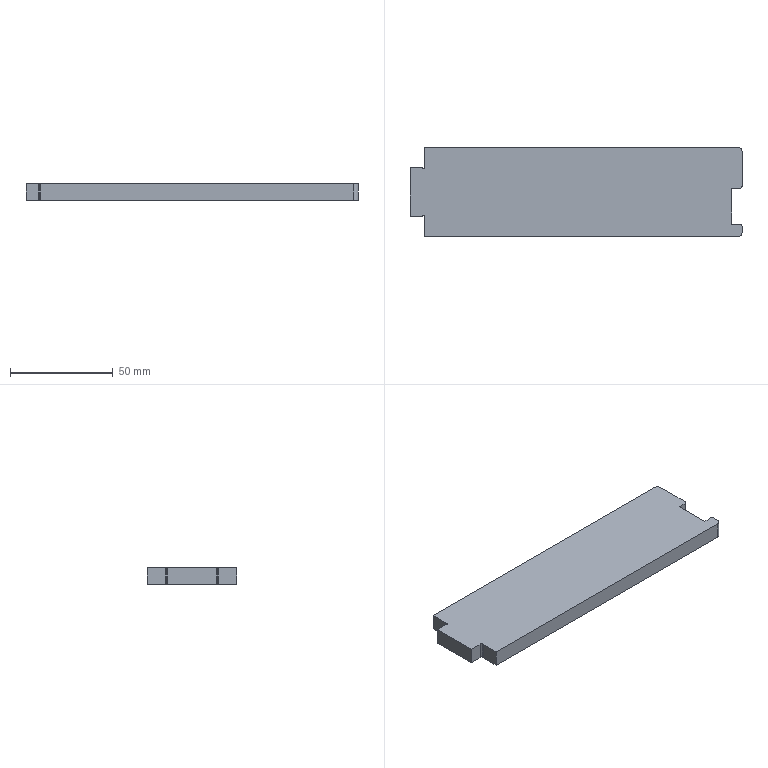Part | SolidWorks | features Fillet 2, FlatPattern 1, ICE 1, SMBaseFlange 1, SheetMetal 1 | 1 solid | 24 faces | box 161.8 x 43.5 x 8 mm | volume 54464 mm3 | plane 14 | cylinder 10 | commonest cylinder face diameters 2 x6 1 x2 4 x2
STEP:
#1=CARTESIAN_POINT('',(-162.8,318.921,0.));
#2=VERTEX_POINT('',#1);
#3=CARTESIAN_POINT('',(-162.8,310.,0.));
#4=VERTEX_POINT('',#3);
#5=CARTESIAN_POINT('',(-162.8,320.,0.));
#6=DIRECTION('',(0.,-1.,0.));
#7=VECTOR('',#6,1000.);
#8=LINE('',#5,#7);
#9=EDGE_CURVE('',#2,#4,#8,.T.);
#10=ORIENTED_EDGE('',*,*,#9,.F.);
#11=CARTESIAN_POINT('',(-162.8,318.921,-8.));
#12=VERTEX_POINT('',#11);
#13=CARTESIAN_POINT('',(-162.8,318.921,-8.));
#14=DIRECTION('',(0.,0.,-1.));
#15=VECTOR('',#14,1000.);
#16=LINE('',#13,#15);
#17=EDGE_CURVE('',#2,#12,#16,.T.);
#18=ORIENTED_EDGE('',*,*,#17,.T.);
#19=CARTESIAN_POINT('',(-162.8,310.,-8.));
#20=VERTEX_POINT('',#19);
#21=CARTESIAN_POINT('',(-162.8,320.,-8.));
#22=DIRECTION('',(0.,-1.,0.));
#23=VECTOR('',#22,1000.);
#24=LINE('',#21,#23);
#25=EDGE_CURVE('',#12,#20,#24,.T.);
#26=ORIENTED_EDGE('',*,*,#25,.T.);
#27=CARTESIAN_POINT('',(-162.8,310.,-8.));
#28=DIRECTION('',(0.,0.,1.));
#29=VECTOR('',#28,1000.);
#30=LINE('',#27,#29);
#31=EDGE_CURVE('',#20,#4,#30,.T.);
#32=ORIENTED_EDGE('',*,*,#31,.T.);
#33=EDGE_LOOP('',(#10,#18,#26,#32));
#34=FACE_OUTER_BOUND('',#33,.T.);
#35=CARTESIAN_POINT('',(-162.8,320.,-8.));
#36=DIRECTION('',(-1.,0.,0.));
#37=DIRECTION('',(0.,0.,1.));
#38=AXIS2_PLACEMENT_3D('',#35,#36,#37);
#39=PLANE('',#38);
#40=ADVANCED_FACE('',(#34),#39,.T.);
#41=CARTESIAN_POINT('',(-169.8,320.,-8.));
#42=VERTEX_POINT('',#41);
#43=CARTESIAN_POINT('',(-163.879,320.,-8.));
#44=VERTEX_POINT('',#43);
#45=CARTESIAN_POINT('',(-162.8,320.,-8.));
#46=DIRECTION('',(1.,0.,0.));
#47=VECTOR('',#46,1000.);
#48=LINE('',#45,#47);
#49=EDGE_CURVE('',#42,#44,#48,.T.);
#50=ORIENTED_EDGE('',*,*,#49,.T.);
#51=CARTESIAN_POINT('',(-163.879,320.,0.));
#52=VERTEX_POINT('',#51);
#53=CARTESIAN_POINT('',(-163.879,320.,-8.));
#54=DIRECTION('',(0.,0.,1.));
#55=VECTOR('',#54,1000.);
#56=LINE('',#53,#55);
#57=EDGE_CURVE('',#44,#52,#56,.T.);
#58=ORIENTED_EDGE('',*,*,#57,.T.);
#59=CARTESIAN_POINT('',(-169.8,320.,0.));
#60=VERTEX_POINT('',#59);
#61=CARTESIAN_POINT('',(-162.8,320.,0.));
#62=DIRECTION('',(1.,0.,0.));
#63=VECTOR('',#62,1000.);
#64=LINE('',#61,#63);
#65=EDGE_CURVE('',#60,#52,#64,.T.);
#66=ORIENTED_EDGE('',*,*,#65,.F.);
#67=CARTESIAN_POINT('',(-169.8,320.,-8.));
#68=DIRECTION('',(0.,0.,1.));
#69=VECTOR('',#68,1000.);
#70=LINE('',#67,#69);
#71=EDGE_CURVE('',#42,#60,#70,.T.);
#72=ORIENTED_EDGE('',*,*,#71,.F.);
#73=EDGE_LOOP('',(#50,#58,#66,#72));
#74=FACE_OUTER_BOUND('',#73,.T.);
#75=CARTESIAN_POINT('',(-162.8,320.,-8.));
#76=DIRECTION('',(0.,-1.,0.));
#77=DIRECTION('',(0.,0.,-1.));
#78=AXIS2_PLACEMENT_3D('',#75,#76,#77);
#79=PLANE('',#78);
#80=ADVANCED_FACE('',(#74),#79,.T.);
#81=CARTESIAN_POINT('',(-163.879,343.5,0.));
#82=VERTEX_POINT('',#81);
#83=CARTESIAN_POINT('',(-169.8,343.5,0.));
#84=VERTEX_POINT('',#83);
#85=CARTESIAN_POINT('',(-169.8,343.5,0.));
#86=DIRECTION('',(-1.,0.,0.));
#87=VECTOR('',#86,1000.);
#88=LINE('',#85,#87);
#89=EDGE_CURVE('',#82,#84,#88,.T.);
#90=ORIENTED_EDGE('',*,*,#89,.F.);
#91=CARTESIAN_POINT('',(-163.879,343.5,-8.));
#92=VERTEX_POINT('',#91);
#93=CARTESIAN_POINT('',(-163.879,343.5,-8.));
#94=DIRECTION('',(0.,0.,-1.));
#95=VECTOR('',#94,1000.);
#96=LINE('',#93,#95);
#97=EDGE_CURVE('',#82,#92,#96,.T.);
#98=ORIENTED_EDGE('',*,*,#97,.T.);
#99=CARTESIAN_POINT('',(-169.8,343.5,-8.));
#100=VERTEX_POINT('',#99);
#101=CARTESIAN_POINT('',(-169.8,343.5,-8.));
#102=DIRECTION('',(-1.,0.,0.));
#103=VECTOR('',#102,1000.);
#104=LINE('',#101,#103);
#105=EDGE_CURVE('',#92,#100,#104,.T.);
#106=ORIENTED_EDGE('',*,*,#105,.T.);
#107=CARTESIAN_POINT('',(-169.8,343.5,-8.));
#108=DIRECTION('',(0.,0.,1.));
#109=VECTOR('',#108,1000.);
#110=LINE('',#107,#109);
#111=EDGE_CURVE('',#100,#84,#110,.T.);
#112=ORIENTED_EDGE('',*,*,#111,.T.);
#113=EDGE_LOOP('',(#90,#98,#106,#112));
#114=FACE_OUTER_BOUND('',#113,.T.);
#115=CARTESIAN_POINT('',(-169.8,343.5,-8.));
#116=DIRECTION('',(0.,1.,0.));
#117=DIRECTION('',(0.,0.,1.));
#118=AXIS2_PLACEMENT_3D('',#115,#116,#117);
#119=PLANE('',#118);
#120=ADVANCED_FACE('',(#114),#119,.T.);
#121=CARTESIAN_POINT('',(-162.8,353.5,-8.));
#122=VERTEX_POINT('',#121);
#123=CARTESIAN_POINT('',(-162.8,344.579,-8.));
#124=VERTEX_POINT('',#123);
#125=CARTESIAN_POINT('',(-162.8,353.5,-8.));
#126=DIRECTION('',(0.,-1.,0.));
#127=VECTOR('',#126,1000.);
#128=LINE('',#125,#127);
#129=EDGE_CURVE('',#122,#124,#128,.T.);
#130=ORIENTED_EDGE('',*,*,#129,.T.);
#131=CARTESIAN_POINT('',(-162.8,344.579,0.));
#132=VERTEX_POINT('',#131);
#133=CARTESIAN_POINT('',(-162.8,344.579,-8.));
#134=DIRECTION('',(0.,0.,1.));
#135=VECTOR('',#134,1000.);
#136=LINE('',#133,#135);
#137=EDGE_CURVE('',#124,#132,#136,.T.);
#138=ORIENTED_EDGE('',*,*,#137,.T.);
#139=CARTESIAN_POINT('',(-162.8,353.5,0.));
#140=VERTEX_POINT('',#139);
#141=CARTESIAN_POINT('',(-162.8,353.5,0.));
#142=DIRECTION('',(0.,-1.,0.));
#143=VECTOR('',#142,1000.);
#144=LINE('',#141,#143);
#145=EDGE_CURVE('',#140,#132,#144,.T.);
#146=ORIENTED_EDGE('',*,*,#145,.F.);
#147=CARTESIAN_POINT('',(-162.8,353.5,-8.));
#148=DIRECTION('',(0.,0.,1.));
#149=VECTOR('',#148,1000.);
#150=LINE('',#147,#149);
#151=EDGE_CURVE('',#122,#140,#150,.T.);
#152=ORIENTED_EDGE('',*,*,#151,.F.);
#153=EDGE_LOOP('',(#130,#138,#146,#152));
#154=FACE_OUTER_BOUND('',#153,.T.);
#155=CARTESIAN_POINT('',(-162.8,353.5,-8.));
#156=DIRECTION('',(-1.,0.,0.));
#157=DIRECTION('',(0.,0.,1.));
#158=AXIS2_PLACEMENT_3D('',#155,#156,#157);
#159=PLANE('',#158);
#160=ADVANCED_FACE('',(#154),#159,.T.);
#161=CARTESIAN_POINT('',(-8.,312.,0.));
#162=VERTEX_POINT('',#161);
#163=CARTESIAN_POINT('',(-8.,315.,0.));
#164=VERTEX_POINT('',#163);
#165=CARTESIAN_POINT('',(-8.,316.,0.));
#166=DIRECTION('',(0.,1.,0.));
#167=VECTOR('',#166,1000.);
#168=LINE('',#165,#167);
#169=EDGE_CURVE('',#162,#164,#168,.T.);
#170=ORIENTED_EDGE('',*,*,#169,.F.);
#171=CARTESIAN_POINT('',(-8.,312.,-8.));
#172=VERTEX_POINT('',#171);
#173=CARTESIAN_POINT('',(-8.,312.,-8.));
#174=DIRECTION('',(0.,0.,-1.));
#175=VECTOR('',#174,1000.);
#176=LINE('',#173,#175);
#177=EDGE_CURVE('',#162,#172,#176,.T.);
#178=ORIENTED_EDGE('',*,*,#177,.T.);
#179=CARTESIAN_POINT('',(-8.,315.,-8.));
#180=VERTEX_POINT('',#179);
#181=CARTESIAN_POINT('',(-8.,316.,-8.));
#182=DIRECTION('',(0.,1.,0.));
#183=VECTOR('',#182,1000.);
#184=LINE('',#181,#183);
#185=EDGE_CURVE('',#172,#180,#184,.T.);
#186=ORIENTED_EDGE('',*,*,#185,.T.);
#187=CARTESIAN_POINT('',(-8.,315.,-8.));
#188=DIRECTION('',(0.,0.,1.));
#189=VECTOR('',#188,1000.);
#190=LINE('',#187,#189);
#191=EDGE_CURVE('',#180,#164,#190,.T.);
#192=ORIENTED_EDGE('',*,*,#191,.T.);
#193=EDGE_LOOP('',(#170,#178,#186,#192));
#194=FACE_OUTER_BOUND('',#193,.T.);
#195=CARTESIAN_POINT('',(-8.,316.,-8.));
#196=DIRECTION('',(1.,0.,0.));
#197=DIRECTION('',(0.,0.,-1.));
#198=AXIS2_PLACEMENT_3D('',#195,#196,#197);
#199=PLANE('',#198);
#200=ADVANCED_FACE('',(#194),#199,.T.);
#201=CARTESIAN_POINT('',(-10.,310.,-8.));
#202=VERTEX_POINT('',#201);
#203=CARTESIAN_POINT('',(-8.,310.,-8.));
#204=DIRECTION('',(1.,0.,0.));
#205=VECTOR('',#204,1000.);
#206=LINE('',#203,#205);
#207=EDGE_CURVE('',#20,#202,#206,.T.);
#208=ORIENTED_EDGE('',*,*,#207,.T.);
#209=CARTESIAN_POINT('',(-10.,310.,0.));
#210=VERTEX_POINT('',#209);
#211=CARTESIAN_POINT('',(-10.,310.,-8.));
#212=DIRECTION('',(0.,0.,1.));
#213=VECTOR('',#212,1000.);
#214=LINE('',#211,#213);
#215=EDGE_CURVE('',#202,#210,#214,.T.);
#216=ORIENTED_EDGE('',*,*,#215,.T.);
#217=CARTESIAN_POINT('',(-8.,310.,0.));
#218=DIRECTION('',(1.,0.,0.));
#219=VECTOR('',#218,1000.);
#220=LINE('',#217,#219);
#221=EDGE_CURVE('',#4,#210,#220,.T.);
#222=ORIENTED_EDGE('',*,*,#221,.F.);
#223=ORIENTED_EDGE('',*,*,#31,.F.);
#224=EDGE_LOOP('',(#208,#216,#222,#223));
#225=FACE_OUTER_BOUND('',#224,.T.);
#226=CARTESIAN_POINT('',(-8.,310.,-8.));
#227=DIRECTION('',(0.,-1.,0.));
#228=DIRECTION('',(0.,0.,-1.));
#229=AXIS2_PLACEMENT_3D('',#226,#227,#228);
#230=PLANE('',#229);
#231=ADVANCED_FACE('',(#225),#230,.T.);
#232=CARTESIAN_POINT('',(-169.8,320.,0.));
#233=DIRECTION('',(0.,-1.,0.));
#234=VECTOR('',#233,1000.);
#235=LINE('',#232,#234);
#236=EDGE_CURVE('',#84,#60,#235,.T.);
#237=ORIENTED_EDGE('',*,*,#236,.F.);
#238=ORIENTED_EDGE('',*,*,#111,.F.);
#239=CARTESIAN_POINT('',(-169.8,320.,-8.));
#240=DIRECTION('',(0.,-1.,0.));
#241=VECTOR('',#240,1000.);
#242=LINE('',#239,#241);
#243=EDGE_CURVE('',#100,#42,#242,.T.);
#244=ORIENTED_EDGE('',*,*,#243,.T.);
#245=ORIENTED_EDGE('',*,*,#71,.T.);
#246=EDGE_LOOP('',(#237,#238,#244,#245));
#247=FACE_OUTER_BOUND('',#246,.T.);
#248=CARTESIAN_POINT('',(-169.8,320.,-8.));
#249=DIRECTION('',(-1.,0.,0.));
#250=DIRECTION('',(0.,0.,1.));
#251=AXIS2_PLACEMENT_3D('',#248,#249,#250);
#252=PLANE('',#251);
#253=ADVANCED_FACE('',(#247),#252,.T.);
#254=CARTESIAN_POINT('',(-10.,353.5,0.));
#255=VERTEX_POINT('',#254);
#256=CARTESIAN_POINT('',(-8.,353.5,0.));
#257=DIRECTION('',(-1.,0.,0.));
#258=VECTOR('',#257,1000.);
#259=LINE('',#256,#258);
#260=EDGE_CURVE('',#255,#140,#259,.T.);
#261=ORIENTED_EDGE('',*,*,#260,.F.);
#262=CARTESIAN_POINT('',(-10.,353.5,-8.));
#263=VERTEX_POINT('',#262);
#264=CARTESIAN_POINT('',(-10.,353.5,-8.));
#265=DIRECTION('',(0.,0.,-1.));
#266=VECTOR('',#265,1000.);
#267=LINE('',#264,#266);
#268=EDGE_CURVE('',#255,#263,#267,.T.);
#269=ORIENTED_EDGE('',*,*,#268,.T.);
#270=CARTESIAN_POINT('',(-8.,353.5,-8.));
#271=DIRECTION('',(-1.,0.,0.));
#272=VECTOR('',#271,1000.);
#273=LINE('',#270,#272);
#274=EDGE_CURVE('',#263,#122,#273,.T.);
#275=ORIENTED_EDGE('',*,*,#274,.T.);
#276=ORIENTED_EDGE('',*,*,#151,.T.);
#277=EDGE_LOOP('',(#261,#269,#275,#276));
#278=FACE_OUTER_BOUND('',#277,.T.);
#279=CARTESIAN_POINT('',(-8.,353.5,-8.));
#280=DIRECTION('',(0.,1.,0.));
#281=DIRECTION('',(0.,0.,1.));
#282=AXIS2_PLACEMENT_3D('',#279,#280,#281);
#283=PLANE('',#282);
#284=ADVANCED_FACE('',(#278),#283,.T.);
#285=CARTESIAN_POINT('',(-8.,334.5,-8.));
#286=VERTEX_POINT('',#285);
#287=CARTESIAN_POINT('',(-8.,351.5,-8.));
#288=VERTEX_POINT('',#287);
#289=CARTESIAN_POINT('',(-8.,333.5,-8.));
#290=DIRECTION('',(0.,1.,0.));
#291=VECTOR('',#290,1000.);
#292=LINE('',#289,#291);
#293=EDGE_CURVE('',#286,#288,#292,.T.);
#294=ORIENTED_EDGE('',*,*,#293,.T.);
#295=CARTESIAN_POINT('',(-8.,351.5,0.));
#296=VERTEX_POINT('',#295);
#297=CARTESIAN_POINT('',(-8.,351.5,-8.));
#298=DIRECTION('',(0.,0.,1.));
#299=VECTOR('',#298,1000.);
#300=LINE('',#297,#299);
#301=EDGE_CURVE('',#288,#296,#300,.T.);
#302=ORIENTED_EDGE('',*,*,#301,.T.);
#303=CARTESIAN_POINT('',(-8.,334.5,0.));
#304=VERTEX_POINT('',#303);
#305=CARTESIAN_POINT('',(-8.,333.5,0.));
#306=DIRECTION('',(0.,1.,0.));
#307=VECTOR('',#306,1000.);
#308=LINE('',#305,#307);
#309=EDGE_CURVE('',#304,#296,#308,.T.);
#310=ORIENTED_EDGE('',*,*,#309,.F.);
#311=CARTESIAN_POINT('',(-8.,334.5,-8.));
#312=DIRECTION('',(0.,0.,-1.));
#313=VECTOR('',#312,1000.);
#314=LINE('',#311,#313);
#315=EDGE_CURVE('',#304,#286,#314,.T.);
#316=ORIENTED_EDGE('',*,*,#315,.T.);
#317=EDGE_LOOP('',(#294,#302,#310,#316));
#318=FACE_OUTER_BOUND('',#317,.T.);
#319=CARTESIAN_POINT('',(-8.,333.5,-8.));
#320=DIRECTION('',(1.,0.,0.));
#321=DIRECTION('',(0.,0.,-1.));
#322=AXIS2_PLACEMENT_3D('',#319,#320,#321);
#323=PLANE('',#322);
#324=ADVANCED_FACE('',(#318),#323,.T.);
#325=CARTESIAN_POINT('',(-13.,333.5,-8.));
#326=VERTEX_POINT('',#325);
#327=CARTESIAN_POINT('',(-9.,333.5,-8.));
#328=VERTEX_POINT('',#327);
#329=CARTESIAN_POINT('',(-13.,333.5,-8.));
#330=DIRECTION('',(1.,0.,0.));
#331=VECTOR('',#330,1000.);
#332=LINE('',#329,#331);
#333=EDGE_CURVE('',#326,#328,#332,.T.);
#334=ORIENTED_EDGE('',*,*,#333,.T.);
#335=CARTESIAN_POINT('',(-9.,333.5,0.));
#336=VERTEX_POINT('',#335);
#337=CARTESIAN_POINT('',(-9.,333.5,-8.));
#338=DIRECTION('',(0.,0.,1.));
#339=VECTOR('',#338,1000.);
#340=LINE('',#337,#339);
#341=EDGE_CURVE('',#328,#336,#340,.T.);
#342=ORIENTED_EDGE('',*,*,#341,.T.);
#343=CARTESIAN_POINT('',(-13.,333.5,0.));
#344=VERTEX_POINT('',#343);
#345=CARTESIAN_POINT('',(-13.,333.5,0.));
#346=DIRECTION('',(1.,0.,0.));
#347=VECTOR('',#346,1000.);
#348=LINE('',#345,#347);
#349=EDGE_CURVE('',#344,#336,#348,.T.);
#350=ORIENTED_EDGE('',*,*,#349,.F.);
#351=CARTESIAN_POINT('',(-13.,333.5,-8.));
#352=DIRECTION('',(0.,0.,1.));
#353=VECTOR('',#352,1000.);
#354=LINE('',#351,#353);
#355=EDGE_CURVE('',#326,#344,#354,.T.);
#356=ORIENTED_EDGE('',*,*,#355,.F.);
#357=EDGE_LOOP('',(#334,#342,#350,#356));
#358=FACE_OUTER_BOUND('',#357,.T.);
#359=CARTESIAN_POINT('',(-13.,333.5,-8.));
#360=DIRECTION('',(0.,-1.,0.));
#361=DIRECTION('',(0.,0.,-1.));
#362=AXIS2_PLACEMENT_3D('',#359,#360,#361);
#363=PLANE('',#362);
#364=ADVANCED_FACE('',(#358),#363,.T.);
#365=CARTESIAN_POINT('',(-13.,316.,0.));
#366=VERTEX_POINT('',#365);
#367=CARTESIAN_POINT('',(-13.,316.,0.));
#368=DIRECTION('',(0.,1.,0.));
#369=VECTOR('',#368,1000.);
#370=LINE('',#367,#369);
#371=EDGE_CURVE('',#366,#344,#370,.T.);
#372=ORIENTED_EDGE('',*,*,#371,.F.);
#373=CARTESIAN_POINT('',(-13.,316.,-8.));
#374=VERTEX_POINT('',#373);
#375=CARTESIAN_POINT('',(-13.,316.,-8.));
#376=DIRECTION('',(0.,0.,1.));
#377=VECTOR('',#376,1000.);
#378=LINE('',#375,#377);
#379=EDGE_CURVE('',#374,#366,#378,.T.);
#380=ORIENTED_EDGE('',*,*,#379,.F.);
#381=CARTESIAN_POINT('',(-13.,316.,-8.));
#382=DIRECTION('',(0.,1.,0.));
#383=VECTOR('',#382,1000.);
#384=LINE('',#381,#383);
#385=EDGE_CURVE('',#374,#326,#384,.T.);
#386=ORIENTED_EDGE('',*,*,#385,.T.);
#387=ORIENTED_EDGE('',*,*,#355,.T.);
#388=EDGE_LOOP('',(#372,#380,#386,#387));
#389=FACE_OUTER_BOUND('',#388,.T.);
#390=CARTESIAN_POINT('',(-13.,316.,-8.));
#391=DIRECTION('',(1.,0.,0.));
#392=DIRECTION('',(0.,0.,-1.));
#393=AXIS2_PLACEMENT_3D('',#390,#391,#392);
#394=PLANE('',#393);
#395=ADVANCED_FACE('',(#389),#394,.T.);
#396=CARTESIAN_POINT('',(-9.,316.,0.));
#397=VERTEX_POINT('',#396);
#398=CARTESIAN_POINT('',(-8.,316.,0.));
#399=DIRECTION('',(-1.,0.,0.));
#400=VECTOR('',#399,1000.);
#401=LINE('',#398,#400);
#402=EDGE_CURVE('',#397,#366,#401,.T.);
#403=ORIENTED_EDGE('',*,*,#402,.F.);
#404=CARTESIAN_POINT('',(-9.,316.,-8.));
#405=VERTEX_POINT('',#404);
#406=CARTESIAN_POINT('',(-9.,316.,-8.));
#407=DIRECTION('',(0.,0.,-1.));
#408=VECTOR('',#407,1000.);
#409=LINE('',#406,#408);
#410=EDGE_CURVE('',#397,#405,#409,.T.);
#411=ORIENTED_EDGE('',*,*,#410,.T.);
#412=CARTESIAN_POINT('',(-8.,316.,-8.));
#413=DIRECTION('',(-1.,0.,0.));
#414=VECTOR('',#413,1000.);
#415=LINE('',#412,#414);
#416=EDGE_CURVE('',#405,#374,#415,.T.);
#417=ORIENTED_EDGE('',*,*,#416,.T.);
#418=ORIENTED_EDGE('',*,*,#379,.T.);
#419=EDGE_LOOP('',(#403,#411,#417,#418));
#420=FACE_OUTER_BOUND('',#419,.T.);
#421=CARTESIAN_POINT('',(-8.,316.,-8.));
#422=DIRECTION('',(0.,1.,0.));
#423=DIRECTION('',(0.,0.,1.));
#424=AXIS2_PLACEMENT_3D('',#421,#422,#423);
#425=PLANE('',#424);
#426=ADVANCED_FACE('',(#420),#425,.T.);
#427=ORIENTED_EDGE('',*,*,#274,.F.);
#428=CARTESIAN_POINT('',(-10.,351.5,-8.));
#429=DIRECTION('',(0.,0.,-1.));
#430=DIRECTION('',(-1.,0.,0.));
#431=AXIS2_PLACEMENT_3D('',#428,#429,#430);
#432=CIRCLE('',#431,2.);
#433=EDGE_CURVE('',#263,#288,#432,.T.);
#434=ORIENTED_EDGE('',*,*,#433,.T.);
#435=ORIENTED_EDGE('',*,*,#293,.F.);
#436=CARTESIAN_POINT('',(-9.,334.5,-8.));
#437=DIRECTION('',(0.,0.,-1.));
#438=DIRECTION('',(-1.,0.,0.));
#439=AXIS2_PLACEMENT_3D('',#436,#437,#438);
#440=CIRCLE('',#439,1.);
#441=EDGE_CURVE('',#286,#328,#440,.T.);
#442=ORIENTED_EDGE('',*,*,#441,.T.);
#443=ORIENTED_EDGE('',*,*,#333,.F.);
#444=ORIENTED_EDGE('',*,*,#385,.F.);
#445=ORIENTED_EDGE('',*,*,#416,.F.);
#446=CARTESIAN_POINT('',(-9.,315.,-8.));
#447=DIRECTION('',(0.,0.,-1.));
#448=DIRECTION('',(-1.,0.,0.));
#449=AXIS2_PLACEMENT_3D('',#446,#447,#448);
#450=CIRCLE('',#449,1.);
#451=EDGE_CURVE('',#405,#180,#450,.T.);
#452=ORIENTED_EDGE('',*,*,#451,.T.);
#453=ORIENTED_EDGE('',*,*,#185,.F.);
#454=CARTESIAN_POINT('',(-10.,312.,-8.));
#455=DIRECTION('',(0.,0.,-1.));
#456=DIRECTION('',(-1.,0.,0.));
#457=AXIS2_PLACEMENT_3D('',#454,#455,#456);
#458=CIRCLE('',#457,2.);
#459=EDGE_CURVE('',#172,#202,#458,.T.);
#460=ORIENTED_EDGE('',*,*,#459,.T.);
#461=ORIENTED_EDGE('',*,*,#207,.F.);
#462=ORIENTED_EDGE('',*,*,#25,.F.);
#463=CARTESIAN_POINT('',(-162.633,319.474,-8.));
#464=VERTEX_POINT('',#463);
#465=CARTESIAN_POINT('',(-161.8,318.921,-8.));
#466=DIRECTION('',(0.,0.,-1.));
#467=DIRECTION('',(-1.,0.,0.));
#468=AXIS2_PLACEMENT_3D('',#465,#466,#467);
#469=CIRCLE('',#468,1.);
#470=EDGE_CURVE('',#12,#464,#469,.T.);
#471=ORIENTED_EDGE('',*,*,#470,.T.);
#472=CARTESIAN_POINT('',(-163.326,320.167,-8.));
#473=VERTEX_POINT('',#472);
#474=CARTESIAN_POINT('',(-163.05,319.75,-8.));
#475=DIRECTION('',(0.,0.,1.));
#476=DIRECTION('',(1.,0.,0.));
#477=AXIS2_PLACEMENT_3D('',#474,#475,#476);
#478=CIRCLE('',#477,0.5);
#479=EDGE_CURVE('',#464,#473,#478,.T.);
#480=ORIENTED_EDGE('',*,*,#479,.T.);
#481=CARTESIAN_POINT('',(-163.879,321.,-8.));
#482=DIRECTION('',(0.,0.,-1.));
#483=DIRECTION('',(-1.,0.,0.));
#484=AXIS2_PLACEMENT_3D('',#481,#482,#483);
#485=CIRCLE('',#484,1.);
#486=EDGE_CURVE('',#473,#44,#485,.T.);
#487=ORIENTED_EDGE('',*,*,#486,.T.);
#488=ORIENTED_EDGE('',*,*,#49,.F.);
#489=ORIENTED_EDGE('',*,*,#243,.F.);
#490=ORIENTED_EDGE('',*,*,#105,.F.);
#491=CARTESIAN_POINT('',(-163.326,343.333,-8.));
#492=VERTEX_POINT('',#491);
#493=CARTESIAN_POINT('',(-163.879,342.5,-8.));
#494=DIRECTION('',(0.,0.,-1.));
#495=DIRECTION('',(-1.,0.,0.));
#496=AXIS2_PLACEMENT_3D('',#493,#494,#495);
#497=CIRCLE('',#496,1.);
#498=EDGE_CURVE('',#92,#492,#497,.T.);
#499=ORIENTED_EDGE('',*,*,#498,.T.);
#500=CARTESIAN_POINT('',(-162.633,344.026,-8.));
#501=VERTEX_POINT('',#500);
#502=CARTESIAN_POINT('',(-163.05,343.75,-8.));
#503=DIRECTION('',(0.,0.,1.));
#504=DIRECTION('',(1.,0.,0.));
#505=AXIS2_PLACEMENT_3D('',#502,#503,#504);
#506=CIRCLE('',#505,0.5);
#507=EDGE_CURVE('',#492,#501,#506,.T.);
#508=ORIENTED_EDGE('',*,*,#507,.T.);
#509=CARTESIAN_POINT('',(-161.8,344.579,-8.));
#510=DIRECTION('',(0.,0.,-1.));
#511=DIRECTION('',(-1.,0.,0.));
#512=AXIS2_PLACEMENT_3D('',#509,#510,#511);
#513=CIRCLE('',#512,1.);
#514=EDGE_CURVE('',#501,#124,#513,.T.);
#515=ORIENTED_EDGE('',*,*,#514,.T.);
#516=ORIENTED_EDGE('',*,*,#129,.F.);
#517=EDGE_LOOP('',(#427,#434,#435,#442,#443,#444,#445,#452,#453,#460,#461,#462,#471,#480,#487,#488,#489,#490,#499,#508,#515,#516));
#518=FACE_OUTER_BOUND('',#517,.T.);
#519=CARTESIAN_POINT('',(0.,0.,-8.));
#520=DIRECTION('',(0.,0.,-1.));
#521=DIRECTION('',(-1.,0.,0.));
#522=AXIS2_PLACEMENT_3D('',#519,#520,#521);
#523=PLANE('',#522);
#524=ADVANCED_FACE('',(#518),#523,.T.);
#525=ORIENTED_EDGE('',*,*,#309,.T.);
#526=CARTESIAN_POINT('',(-10.,351.5,0.));
#527=DIRECTION('',(0.,0.,1.));
#528=DIRECTION('',(-1.,0.,0.));
#529=AXIS2_PLACEMENT_3D('',#526,#527,#528);
#530=CIRCLE('',#529,2.);
#531=EDGE_CURVE('',#296,#255,#530,.T.);
#532=ORIENTED_EDGE('',*,*,#531,.T.);
#533=ORIENTED_EDGE('',*,*,#260,.T.);
#534=ORIENTED_EDGE('',*,*,#145,.T.);
#535=CARTESIAN_POINT('',(-162.633,344.026,0.));
#536=VERTEX_POINT('',#535);
#537=CARTESIAN_POINT('',(-161.8,344.579,0.));
#538=DIRECTION('',(0.,0.,1.));
#539=DIRECTION('',(-1.,0.,0.));
#540=AXIS2_PLACEMENT_3D('',#537,#538,#539);
#541=CIRCLE('',#540,1.);
#542=EDGE_CURVE('',#132,#536,#541,.T.);
#543=ORIENTED_EDGE('',*,*,#542,.T.);
#544=CARTESIAN_POINT('',(-163.326,343.333,0.));
#545=VERTEX_POINT('',#544);
#546=CARTESIAN_POINT('',(-163.05,343.75,0.));
#547=DIRECTION('',(0.,0.,1.));
#548=DIRECTION('',(1.,0.,0.));
#549=AXIS2_PLACEMENT_3D('',#546,#547,#548);
#550=CIRCLE('',#549,0.5);
#551=EDGE_CURVE('',#545,#536,#550,.T.);
#552=ORIENTED_EDGE('',*,*,#551,.F.);
#553=CARTESIAN_POINT('',(-163.879,342.5,0.));
#554=DIRECTION('',(0.,0.,1.));
#555=DIRECTION('',(-1.,0.,0.));
#556=AXIS2_PLACEMENT_3D('',#553,#554,#555);
#557=CIRCLE('',#556,1.);
#558=EDGE_CURVE('',#545,#82,#557,.T.);
#559=ORIENTED_EDGE('',*,*,#558,.T.);
#560=ORIENTED_EDGE('',*,*,#89,.T.);
#561=ORIENTED_EDGE('',*,*,#236,.T.);
#562=ORIENTED_EDGE('',*,*,#65,.T.);
#563=CARTESIAN_POINT('',(-163.326,320.167,0.));
#564=VERTEX_POINT('',#563);
#565=CARTESIAN_POINT('',(-163.879,321.,0.));
#566=DIRECTION('',(0.,0.,1.));
#567=DIRECTION('',(-1.,0.,0.));
#568=AXIS2_PLACEMENT_3D('',#565,#566,#567);
#569=CIRCLE('',#568,1.);
#570=EDGE_CURVE('',#52,#564,#569,.T.);
#571=ORIENTED_EDGE('',*,*,#570,.T.);
#572=CARTESIAN_POINT('',(-162.633,319.474,0.));
#573=VERTEX_POINT('',#572);
#574=CARTESIAN_POINT('',(-163.05,319.75,0.));
#575=DIRECTION('',(0.,0.,1.));
#576=DIRECTION('',(1.,0.,0.));
#577=AXIS2_PLACEMENT_3D('',#574,#575,#576);
#578=CIRCLE('',#577,0.5);
#579=EDGE_CURVE('',#573,#564,#578,.T.);
#580=ORIENTED_EDGE('',*,*,#579,.F.);
#581=CARTESIAN_POINT('',(-161.8,318.921,0.));
#582=DIRECTION('',(0.,0.,1.));
#583=DIRECTION('',(-1.,0.,0.));
#584=AXIS2_PLACEMENT_3D('',#581,#582,#583);
#585=CIRCLE('',#584,1.);
#586=EDGE_CURVE('',#573,#2,#585,.T.);
#587=ORIENTED_EDGE('',*,*,#586,.T.);
#588=ORIENTED_EDGE('',*,*,#9,.T.);
#589=ORIENTED_EDGE('',*,*,#221,.T.);
#590=CARTESIAN_POINT('',(-10.,312.,0.));
#591=DIRECTION('',(0.,0.,1.));
#592=DIRECTION('',(-1.,0.,0.));
#593=AXIS2_PLACEMENT_3D('',#590,#591,#592);
#594=CIRCLE('',#593,2.);
#595=EDGE_CURVE('',#210,#162,#594,.T.);
#596=ORIENTED_EDGE('',*,*,#595,.T.);
#597=ORIENTED_EDGE('',*,*,#169,.T.);
#598=CARTESIAN_POINT('',(-9.,315.,0.));
#599=DIRECTION('',(0.,0.,1.));
#600=DIRECTION('',(-1.,0.,0.));
#601=AXIS2_PLACEMENT_3D('',#598,#599,#600);
#602=CIRCLE('',#601,1.);
#603=EDGE_CURVE('',#164,#397,#602,.T.);
#604=ORIENTED_EDGE('',*,*,#603,.T.);
#605=ORIENTED_EDGE('',*,*,#402,.T.);
#606=ORIENTED_EDGE('',*,*,#371,.T.);
#607=ORIENTED_EDGE('',*,*,#349,.T.);
#608=CARTESIAN_POINT('',(-9.,334.5,0.));
#609=DIRECTION('',(0.,0.,1.));
#610=DIRECTION('',(-1.,0.,0.));
#611=AXIS2_PLACEMENT_3D('',#608,#609,#610);
#612=CIRCLE('',#611,1.);
#613=EDGE_CURVE('',#336,#304,#612,.T.);
#614=ORIENTED_EDGE('',*,*,#613,.T.);
#615=EDGE_LOOP('',(#525,#532,#533,#534,#543,#552,#559,#560,#561,#562,#571,#580,#587,#588,#589,#596,#597,#604,#605,#606,#607,#614));
#616=FACE_OUTER_BOUND('',#615,.T.);
#617=CARTESIAN_POINT('',(0.,0.,0.));
#618=DIRECTION('',(0.,0.,-1.));
#619=DIRECTION('',(-1.,0.,0.));
#620=AXIS2_PLACEMENT_3D('',#617,#618,#619);
#621=PLANE('',#620);
#622=ADVANCED_FACE('',(#616),#621,.F.);
#623=ORIENTED_EDGE('',*,*,#579,.T.);
#624=CARTESIAN_POINT('',(-163.326,320.167,-8.));
#625=DIRECTION('',(0.,0.,-1.));
#626=VECTOR('',#625,1000.);
#627=LINE('',#624,#626);
#628=EDGE_CURVE('',#564,#473,#627,.T.);
#629=ORIENTED_EDGE('',*,*,#628,.T.);
#630=ORIENTED_EDGE('',*,*,#479,.F.);
#631=CARTESIAN_POINT('',(-162.633,319.474,-8.));
#632=DIRECTION('',(0.,0.,1.));
#633=VECTOR('',#632,1000.);
#634=LINE('',#631,#633);
#635=EDGE_CURVE('',#464,#573,#634,.T.);
#636=ORIENTED_EDGE('',*,*,#635,.T.);
#637=EDGE_LOOP('',(#623,#629,#630,#636));
#638=FACE_OUTER_BOUND('',#637,.T.);
#639=CARTESIAN_POINT('',(-163.05,319.75,-8.));
#640=DIRECTION('',(0.,0.,-1.));
#641=DIRECTION('',(-1.,0.,0.));
#642=AXIS2_PLACEMENT_3D('',#639,#640,#641);
#643=CYLINDRICAL_SURFACE('',#642,0.5);
#644=ADVANCED_FACE('',(#638),#643,.F.);
#645=ORIENTED_EDGE('',*,*,#507,.F.);
#646=CARTESIAN_POINT('',(-163.326,343.333,-8.));
#647=DIRECTION('',(0.,0.,1.));
#648=VECTOR('',#647,1000.);
#649=LINE('',#646,#648);
#650=EDGE_CURVE('',#492,#545,#649,.T.);
#651=ORIENTED_EDGE('',*,*,#650,.T.);
#652=ORIENTED_EDGE('',*,*,#551,.T.);
#653=CARTESIAN_POINT('',(-162.633,344.026,-8.));
#654=DIRECTION('',(0.,0.,-1.));
#655=VECTOR('',#654,1000.);
#656=LINE('',#653,#655);
#657=EDGE_CURVE('',#536,#501,#656,.T.);
#658=ORIENTED_EDGE('',*,*,#657,.T.);
#659=EDGE_LOOP('',(#645,#651,#652,#658));
#660=FACE_OUTER_BOUND('',#659,.T.);
#661=CARTESIAN_POINT('',(-163.05,343.75,-8.));
#662=DIRECTION('',(0.,0.,-1.));
#663=DIRECTION('',(-1.,0.,0.));
#664=AXIS2_PLACEMENT_3D('',#661,#662,#663);
#665=CYLINDRICAL_SURFACE('',#664,0.5);
#666=ADVANCED_FACE('',(#660),#665,.F.);
#667=ORIENTED_EDGE('',*,*,#451,.F.);
#668=ORIENTED_EDGE('',*,*,#410,.F.);
#669=ORIENTED_EDGE('',*,*,#603,.F.);
#670=ORIENTED_EDGE('',*,*,#191,.F.);
#671=EDGE_LOOP('',(#667,#668,#669,#670));
#672=FACE_OUTER_BOUND('',#671,.T.);
#673=CARTESIAN_POINT('',(-9.,315.,-8.));
#674=DIRECTION('',(0.,0.,1.));
#675=DIRECTION('',(1.,0.,0.));
#676=AXIS2_PLACEMENT_3D('',#673,#674,#675);
#677=CYLINDRICAL_SURFACE('',#676,1.);
#678=ADVANCED_FACE('',(#672),#677,.T.);
#679=ORIENTED_EDGE('',*,*,#441,.F.);
#680=ORIENTED_EDGE('',*,*,#315,.F.);
#681=ORIENTED_EDGE('',*,*,#613,.F.);
#682=ORIENTED_EDGE('',*,*,#341,.F.);
#683=EDGE_LOOP('',(#679,#680,#681,#682));
#684=FACE_OUTER_BOUND('',#683,.T.);
#685=CARTESIAN_POINT('',(-9.,334.5,-8.));
#686=DIRECTION('',(0.,0.,1.));
#687=DIRECTION('',(1.,0.,0.));
#688=AXIS2_PLACEMENT_3D('',#685,#686,#687);
#689=CYLINDRICAL_SURFACE('',#688,1.);
#690=ADVANCED_FACE('',(#684),#689,.T.);
#691=ORIENTED_EDGE('',*,*,#486,.F.);
#692=ORIENTED_EDGE('',*,*,#628,.F.);
#693=ORIENTED_EDGE('',*,*,#570,.F.);
#694=ORIENTED_EDGE('',*,*,#57,.F.);
#695=EDGE_LOOP('',(#691,#692,#693,#694));
#696=FACE_OUTER_BOUND('',#695,.T.);
#697=CARTESIAN_POINT('',(-163.879,321.,-8.));
#698=DIRECTION('',(0.,0.,-1.));
#699=DIRECTION('',(-1.,0.,0.));
#700=AXIS2_PLACEMENT_3D('',#697,#698,#699);
#701=CYLINDRICAL_SURFACE('',#700,1.);
#702=ADVANCED_FACE('',(#696),#701,.T.);
#703=ORIENTED_EDGE('',*,*,#470,.F.);
#704=ORIENTED_EDGE('',*,*,#17,.F.);
#705=ORIENTED_EDGE('',*,*,#586,.F.);
#706=ORIENTED_EDGE('',*,*,#635,.F.);
#707=EDGE_LOOP('',(#703,#704,#705,#706));
#708=FACE_OUTER_BOUND('',#707,.T.);
#709=CARTESIAN_POINT('',(-161.8,318.921,-8.));
#710=DIRECTION('',(0.,0.,-1.));
#711=DIRECTION('',(-1.,0.,0.));
#712=AXIS2_PLACEMENT_3D('',#709,#710,#711);
#713=CYLINDRICAL_SURFACE('',#712,1.);
#714=ADVANCED_FACE('',(#708),#713,.T.);
#715=ORIENTED_EDGE('',*,*,#498,.F.);
#716=ORIENTED_EDGE('',*,*,#97,.F.);
#717=ORIENTED_EDGE('',*,*,#558,.F.);
#718=ORIENTED_EDGE('',*,*,#650,.F.);
#719=EDGE_LOOP('',(#715,#716,#717,#718));
#720=FACE_OUTER_BOUND('',#719,.T.);
#721=CARTESIAN_POINT('',(-163.879,342.5,-8.));
#722=DIRECTION('',(0.,0.,-1.));
#723=DIRECTION('',(-1.,0.,0.));
#724=AXIS2_PLACEMENT_3D('',#721,#722,#723);
#725=CYLINDRICAL_SURFACE('',#724,1.);
#726=ADVANCED_FACE('',(#720),#725,.T.);
#727=ORIENTED_EDGE('',*,*,#514,.F.);
#728=ORIENTED_EDGE('',*,*,#657,.F.);
#729=ORIENTED_EDGE('',*,*,#542,.F.);
#730=ORIENTED_EDGE('',*,*,#137,.F.);
#731=EDGE_LOOP('',(#727,#728,#729,#730));
#732=FACE_OUTER_BOUND('',#731,.T.);
#733=CARTESIAN_POINT('',(-161.8,344.579,-8.));
#734=DIRECTION('',(0.,0.,-1.));
#735=DIRECTION('',(-1.,0.,0.));
#736=AXIS2_PLACEMENT_3D('',#733,#734,#735);
#737=CYLINDRICAL_SURFACE('',#736,1.);
#738=ADVANCED_FACE('',(#732),#737,.T.);
#739=ORIENTED_EDGE('',*,*,#433,.F.);
#740=ORIENTED_EDGE('',*,*,#268,.F.);
#741=ORIENTED_EDGE('',*,*,#531,.F.);
#742=ORIENTED_EDGE('',*,*,#301,.F.);
#743=EDGE_LOOP('',(#739,#740,#741,#742));
#744=FACE_OUTER_BOUND('',#743,.T.);
#745=CARTESIAN_POINT('',(-10.,351.5,-8.));
#746=DIRECTION('',(0.,0.,1.));
#747=DIRECTION('',(1.,0.,0.));
#748=AXIS2_PLACEMENT_3D('',#745,#746,#747);
#749=CYLINDRICAL_SURFACE('',#748,2.);
#750=ADVANCED_FACE('',(#744),#749,.T.);
#751=ORIENTED_EDGE('',*,*,#459,.F.);
#752=ORIENTED_EDGE('',*,*,#177,.F.);
#753=ORIENTED_EDGE('',*,*,#595,.F.);
#754=ORIENTED_EDGE('',*,*,#215,.F.);
#755=EDGE_LOOP('',(#751,#752,#753,#754));
#756=FACE_OUTER_BOUND('',#755,.T.);
#757=CARTESIAN_POINT('',(-10.,312.,-8.));
#758=DIRECTION('',(0.,0.,1.));
#759=DIRECTION('',(1.,0.,0.));
#760=AXIS2_PLACEMENT_3D('',#757,#758,#759);
#761=CYLINDRICAL_SURFACE('',#760,2.);
#762=ADVANCED_FACE('',(#756),#761,.T.);
#763=CLOSED_SHELL('',(#40,#80,#120,#160,#200,#231,#253,#284,#324,#364,#395,#426,#524,#622,#644,#666,#678,#690,#702,#714,#726,#738,#750,#762));
#764=MANIFOLD_SOLID_BREP('',#763);
#765=CARTESIAN_POINT('',(0.,0.,0.));
#766=DIRECTION('',(0.,0.,1.));
#767=DIRECTION('',(1.,0.,0.));
#768=AXIS2_PLACEMENT_3D('',#765,#766,#767);
#769=(LENGTH_UNIT()NAMED_UNIT(*)SI_UNIT(.MILLI.,.METRE.));
#770=UNCERTAINTY_MEASURE_WITH_UNIT(LENGTH_MEASURE(0.00001),#769,'','');
#771=(NAMED_UNIT(*)PLANE_ANGLE_UNIT()SI_UNIT($,.RADIAN.));
#772=(NAMED_UNIT(*)SI_UNIT($,.STERADIAN.)SOLID_ANGLE_UNIT());
#773=(GEOMETRIC_REPRESENTATION_CONTEXT(3)GLOBAL_UNCERTAINTY_ASSIGNED_CONTEXT((#770))GLOBAL_UNIT_ASSIGNED_CONTEXT((#769,#771,#772))REPRESENTATION_CONTEXT('',''));
#774=ADVANCED_BREP_SHAPE_REPRESENTATION('',(#764,#768),#773);